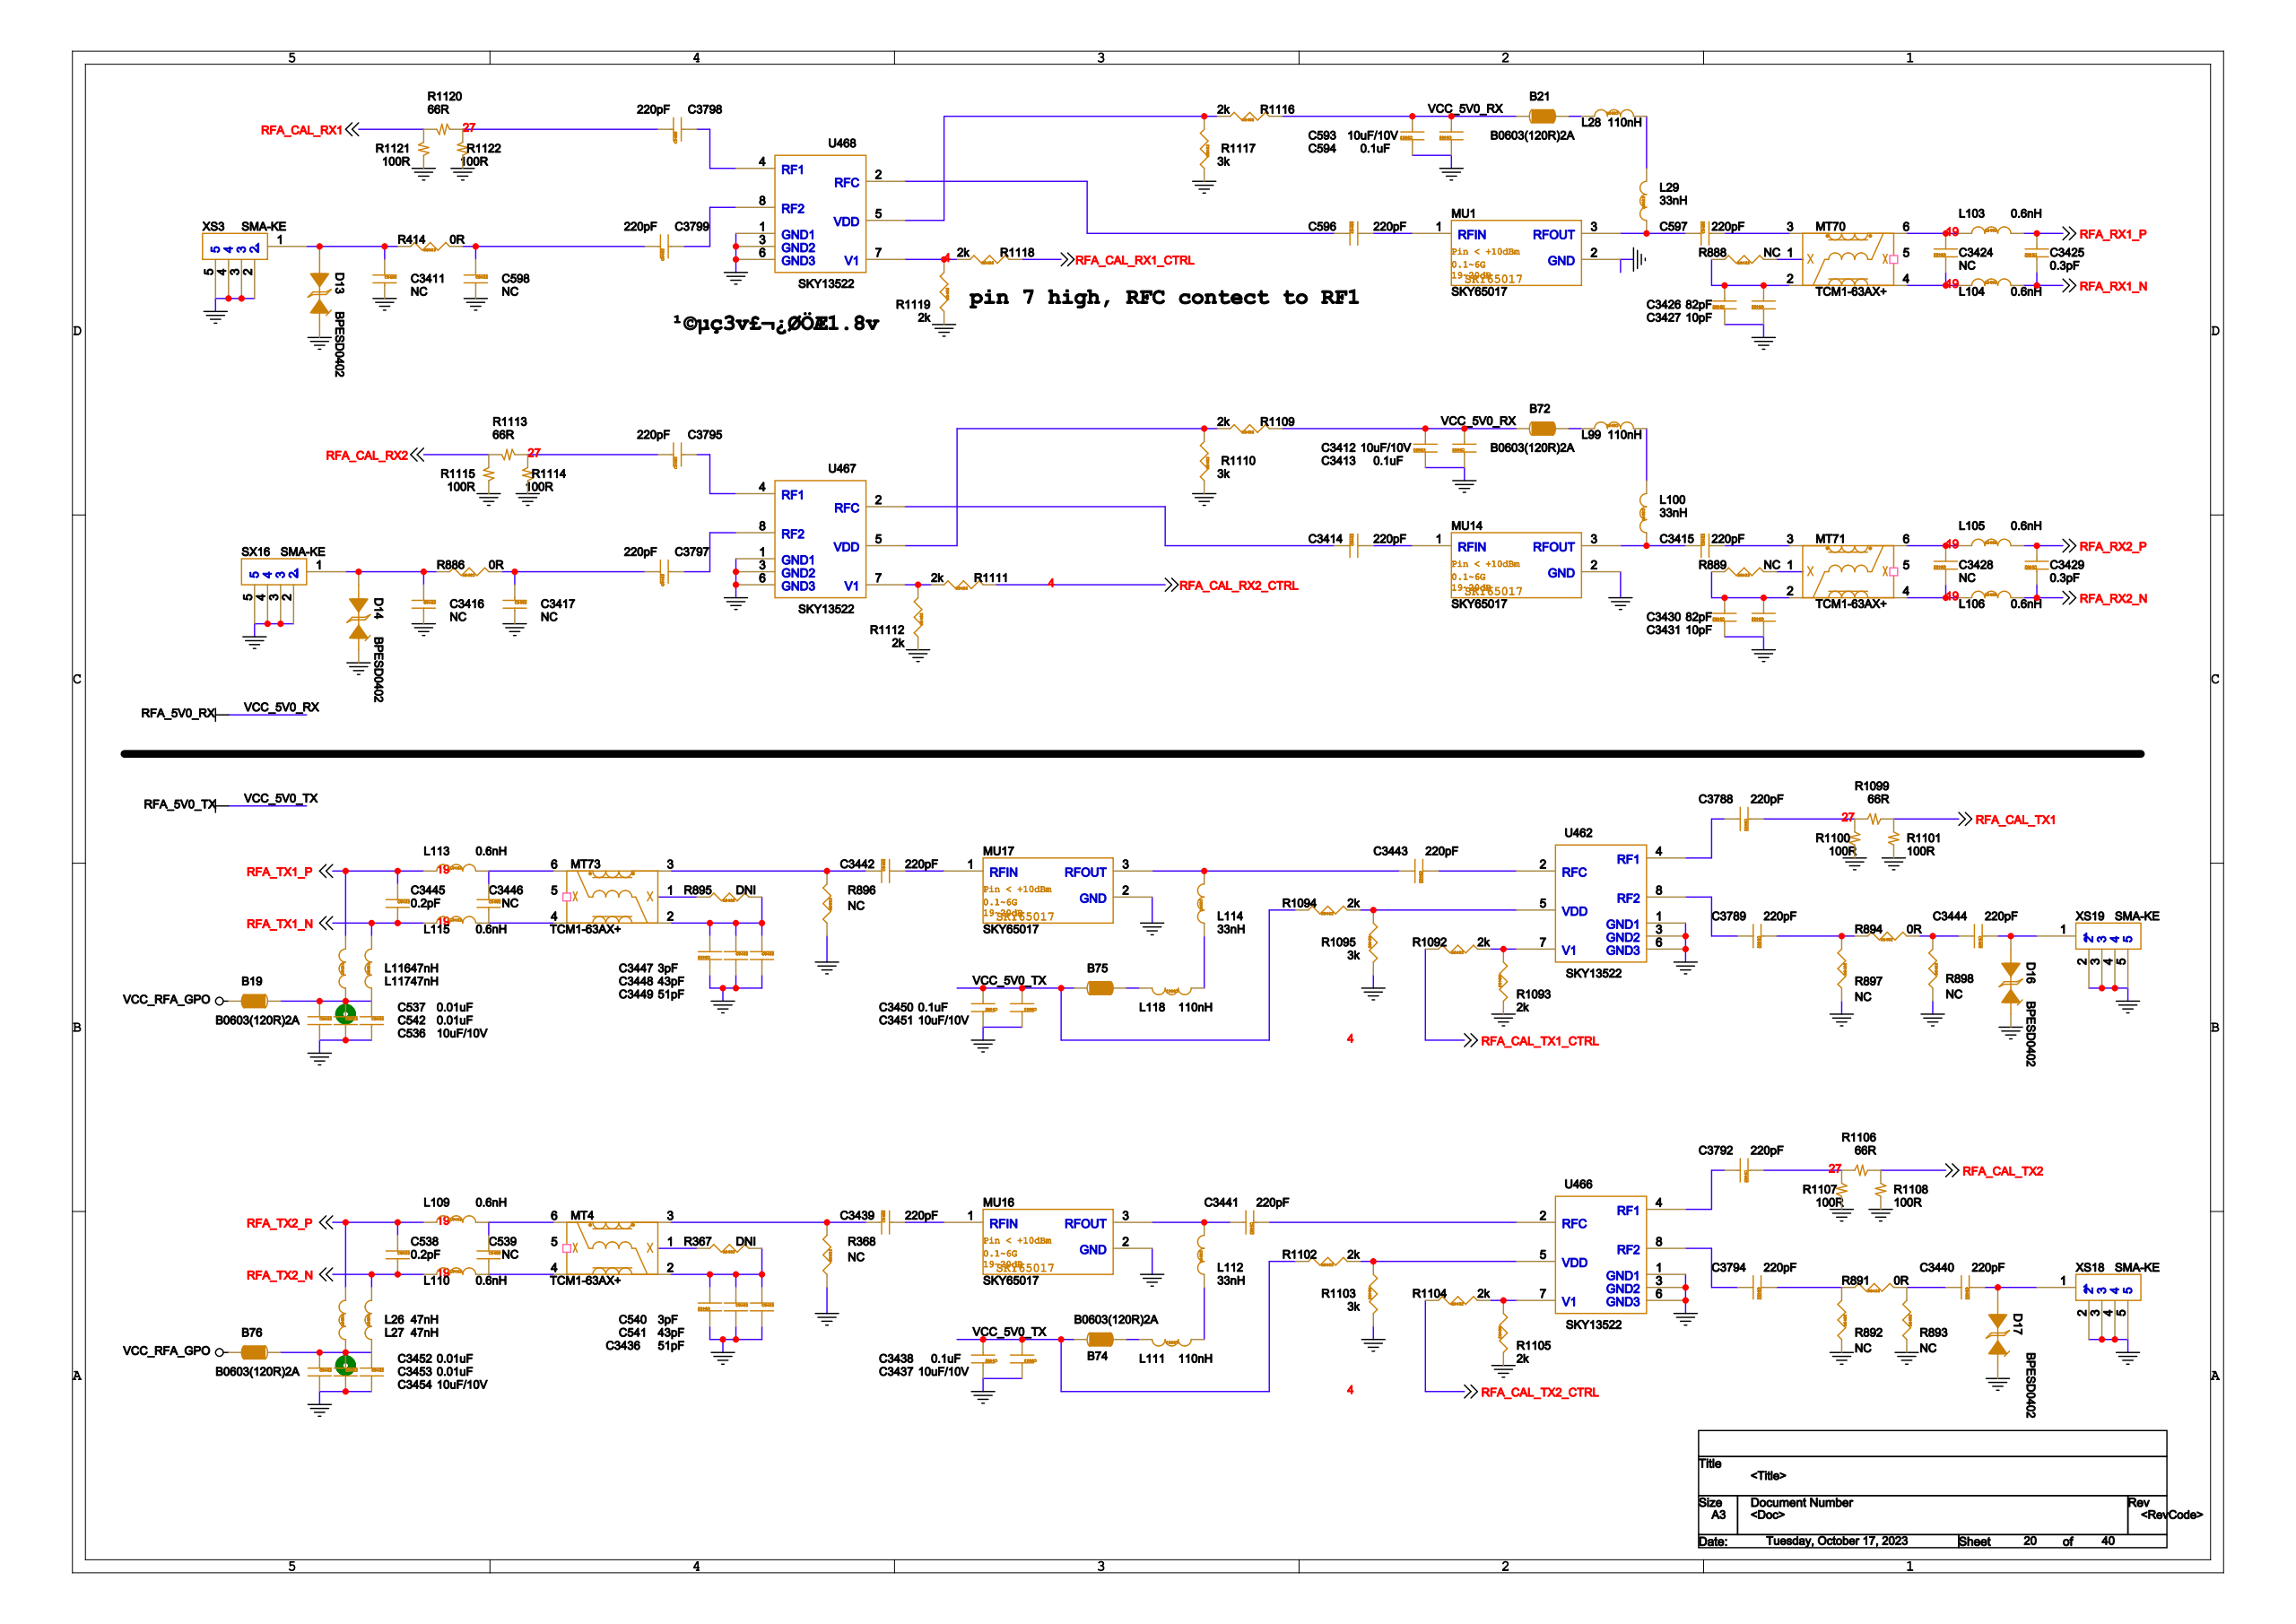Circuit board | Cadence Allegro | 1793 parts | 1223 nets | one sheet of the schematic
Parts on this sheet (reference | value | footprint):
B19 | B0603(120R)2A | B0603
B21 | B0603(120R)2A | B0603
B72 | B0603(120R)2A | B0603
B74 | B0603(120R)2A | B0603
B75 | B0603(120R)2A | B0603
B76 | B0603(120R)2A | B0603
C536 | 10uF/10V | C0402
C537 | 0.01uF | C0402
C538 | 0.2pF | C0402
C539 | NC | C0402
C540 | 3pF | C0402
C541 | 43pF | C0402
C542 | 0.01uF | C0402
C593 | 10uF/10V | C0402
C594 | 0.1uF | C0402
C596 | 220pF | C0402
C597 | 220pF | C0402
C598 | NC | C0402
C3411 | NC | C0402
C3412 | 10uF/10V | C0402
C3413 | 0.1uF | C0402
C3414 | 220pF | C0402
C3415 | 220pF | C0402
C3416 | NC | C0402
C3417 | NC | C0402
C3424 | NC | C0402
C3425 | 0.3pF | C0402
C3426 | 82pF | C0402
C3427 | 10pF | C0402
C3428 | NC | C0402
C3429 | 0.3pF | C0402
C3430 | 82pF | C0402
C3431 | 10pF | C0402
C3436 | 51pF | C0402
C3437 | 10uF/10V | C0402
C3438 | 0.1uF | C0402
C3439 | 220pF | C0402
C3440 | 220pF | C0402
C3441 | 220pF | C0402
C3442 | 220pF | C0402
C3443 | 220pF | C0402
C3444 | 220pF | C0402
C3445 | 0.2pF | C0402
C3446 | NC | C0402
C3447 | 3pF | C0402
C3448 | 43pF | C0402
C3449 | 51pF | C0402
C3450 | 0.1uF | C0402
C3451 | 10uF/10V | C0402
C3452 | 0.01uF | C0402
C3453 | 0.01uF | C0402
C3454 | 10uF/10V | C0402
C3788 | 220pF | C0402
C3789 | 220pF | C0402
C3792 | 220pF | C0402
C3794 | 220pF | C0402
C3795 | 220pF | C0402
C3797 | 220pF | C0402
C3798 | 220pF | C0402
C3799 | 220pF | C0402
D13 | BPESD0402 | C0402
D14 | BPESD0402 | C0402
D16 | BPESD0402 | C0402
D17 | BPESD0402 | C0402
L26 | 47nH | L0603
L27 | 47nH | L0603
L28 | 110nH | L0603
L29 | 33nH | L0603
L99 | 110nH | L0603
L100 | 33nH | L0603
L103 | 0.6nH | L0402
L104 | 0.6nH | L0402
L105 | 0.6nH | L0402
L106 | 0.6nH | L0402
L109 | 0.6nH | L0402
L110 | 0.6nH | L0402
L111 | 110nH | L0603
L112 | 33nH | L0603
L113 | 0.6nH | L0402
L114 | 33nH | L0603
L115 | 0.6nH | L0402
L118 | 110nH | L0603
MT4 | TCM1-63AX+ | TCM1-63AX
MT70 | TCM1-63AX+ | TCM1-63AX
MT71 | TCM1-63AX+ | TCM1-63AX
MT73 | TCM1-63AX+ | TCM1-63AX
MU1 | SKY65017 | SOT89_3
MU14 | SKY65017 | SOT89_3
MU16 | SKY65017 | SOT89_3
MU17 | SKY65017 | SOT89_3
R367 | DNI | R0402
R368 | NC | R0402
R414 | 0R | R0603
R886 | 0R | R0603
R888 | NC | R0402
R889 | NC | R0402
R891 | 0R | R0402
R892 | NC | R0402
R893 | NC | R0402
R894 | 0R | R0402
R895 | DNI | R0402
R896 | NC | R0402
R897 | NC | R0402
R898 | NC | R0402
R1092 | 2k | R0402
R1093 | 2k | R0402
R1094 | 2k | R0402
R1095 | 3k | R0402
R1099 | 66R | R0402
R1100 | 100R | R0402
R1101 | 100R | R0402
R1102 | 2k | R0402
R1103 | 3k | R0402
R1104 | 2k | R0402
R1105 | 2k | R0402
R1106 | 66R | R0402
R1107 | 100R | R0402
R1108 | 100R | R0402
R1109 | 2k | R0402
R1110 | 3k | R0402
R1111 | 2k | R0402
R1112 | 2k | R0402
R1113 | 66R | R0402
R1114 | 100R | R0402
R1115 | 100R | R0402
R1116 | 2k | R0402
R1117 | 3k | R0402
R1118 | 2k | R0402
R1119 | 2k | R0402
R1120 | 66R | R0402
R1121 | 100R | R0402
R1122 | 100R | R0402
SX16 | SMA-KE | SMA-SMD_BWSMA-KE-P001
U462 | SKY13522 | TSNP-8_L1_1-W1_1-P0_40-BL
U466 | SKY13522 | TSNP-8_L1_1-W1_1-P0_40-BL
U467 | SKY13522 | TSNP-8_L1_1-W1_1-P0_40-BL
U468 | SKY13522 | TSNP-8_L1_1-W1_1-P0_40-BL
XS3 | SMA-KE | SMA-SMD_BWSMA-KE-P001
XS18 | SMA-KE | SMA-SMD_BWSMA-KE-P001
XS19 | SMA-KE | SMA-SMD_BWSMA-KE-P001
Nets of these parts (net: part-pin ...):
GND: C536-2 C537-2 C540-1 C541-2 C542-2 C593-1 C594-1 C598-2 C3411-2 C3412-1 C3413-1 C3416-2 C3417-2 C3426-1 C3427-1 C3430-1 C3431-1 C3436-2 C3437-1 C3438-1 C3447-1 C3448-2 C3449-2 C3450-1 C3451-1 C3452-2 C3453-2 C3454-2 D13-2 D14-2 D16-2 D17-2 MU1-2 MU14-2 MU16-2 MU17-2 R368-1 R892-1 R893-1 R896-1 R897-1 R898-1 R1093-2 R1095-2 R1100-1 R1101-1 R1103-2 R1105-2 R1107-1 R1108-1 R1110-2 R1112-2 R1114-1 R1115-1 R1117-2 R1119-2 R1121-1 R1122-1 SX16-2 SX16-3 SX16-4 SX16-5 U462-1 U462-3 U462-6 U466-1 U466-3 U466-6 U467-1 U467-3 U467-6 U468-1 U468-3 U468-6 XS3-2 XS3-3 XS3-4 XS3-5 XS18-2 XS18-3 XS18-4 XS18-5 XS19-2 XS19-3 XS19-4 XS19-5
N17038594: C3411-1 D13-1 R414-1 XS3-1
N17042265: C3416-1 D14-1 R886-1 SX16-1
N17055895: C3444-1 D16-1 XS19-1
N17056237: C3440-1 D17-1 XS18-1
RFA_CAL_TX1_CTRL: R1092-1
N18637396: R1092-2 R1093-1 U462-7
RFA_5V0_TX: B74-1 B75-1 C3437-2 C3438-2 C3450-2 C3451-2 R1094-1 R1102-1
N18612424: R1094-2 R1095-1 U462-5
N18679446: R1102-2 R1103-1 U466-5
RFA_CAL_TX2_CTRL: R1104-1
N18679484: R1104-2 R1105-1 U466-7
RFA_5V0_RX: B21-1 B72-1 C593-2 C594-2 C3412-2 C3413-2 R1109-1 R1116-1
N18681713: R1109-2 R1110-1 U467-5
RFA_CAL_RX2_CTRL: R1111-1
N18681751: R1111-2 R1112-1 U467-7
N18683006: R1116-2 R1117-1 U468-5
RFA_CAL_RX1_CTRL: R1118-1
N18683048: R1118-2 R1119-1 U468-7
N18664130: C3788-1 R1099-1 R1100-2
RFA_CAL_TX1: R1099-2 R1101-2
N18679400: C3792-1 R1106-1 R1107-2
RFA_CAL_TX2: R1106-2 R1108-2
N18681669: C3795-1 R1113-1 R1114-2
RFA_CAL_RX2: R1113-2 R1115-2
N18682970: C3798-1 R1120-1 R1122-2
RFA_CAL_RX1: R1120-2 R1121-2
N18612280: C3788-2 U462-4
N18664648: C3789-2 U462-8
N18612132: C3443-1 U462-2
N18679396: C3792-2 U466-4
N18679438: C3794-2 U466-8
N18679426: C3441-1 U466-2
N18681665: C3795-2 U467-4
N18681707: C3797-2 U467-8
N18681695: C3414-1 U467-2
N18682972: C3798-2 U468-4
N18682994: C3799-2 U468-8
N18682992: C596-1 U468-2
N17056451: B76-1 C3452-1 C3453-1 C3454-1 L26-1 L27-1
N17056106: B19-1 C536-1 C537-1 C542-1
N17038892: C596-2 MU1-1
N1059479: C597-1 L29-2 MU1-3
N17042279: C3414-2 MU14-1
N17042281: C3415-1 L100-2 MU14-3
N17056223: C3439-2 MU16-1
N17056225: C3441-2 L112-1 MU16-3
N17055881: C3442-2 MU17-1
N17055883: C3443-2 L114-1 MU17-3
RFA_RX1_N: C3425-1 L104-2
RFA_RX1_P: C3425-2 L103-2
RFA_RX2_N: C3429-1 L106-2
RFA_RX2_P: C3429-2 L105-2
RFA_TX1_N: C3445-2 L115-1
RFA_TX1_P: C3445-1 L113-1
RFA_TX2_N: C538-2 L27-2 L110-1
RFA_TX2_P: C538-1 L26-2 L109-1
VCC_RFA_GPO: B19-2 B76-2
N17039097: B21-2 L28-2
N17042195: B72-2 L99-2
N17056438: B74-2 L111-2
N17056096: B75-2 L118-2
N17042273: C3417-1 C3797-1 R886-2
N17042946: C3424-1 L104-1 MT70-4
N17042909: C3424-2 L103-1 MT70-6
N17044828: C3428-1 L106-1 MT71-4
N17044794: C3428-2 L105-1 MT71-6
N17055861: C3446-1 L113-2 MT73-6
N17055984: C3446-2 L115-2 MT73-4
N17056203: C539-1 L109-2 MT4-6
N17056326: C539-2 L110-2 MT4-4
N724433: C598-1 C3799-1 R414-2
N17055889: C3789-1 R894-1 R897-2
N17056229: C3794-1 R891-1 R892-2
N17044780: C3415-2 MT71-3
N17056219: C3439-1 MT4-3 R368-2
N17056235: C3440-2 R891-2 R893-2
N17055877: C3442-1 MT73-3 R896-2
N17055891: C3444-2 R894-2 R898-2
N1025474: C597-2 MT70-3
N17042942: C3426-2 C3427-2 MT70-2 R888-1
N17044824: C3430-2 C3431-2 MT71-2 R889-1
N17056301: C540-2 C541-1 C3436-1 MT4-2 R367-2
N17055959: C3447-2 C3448-1 C3449-1 MT73-2 R895-2
N17042197: L99-1 L100-1
N17056344: L111-1 L112-2
N17056002: L114-2 L118-1
N17039045: L28-1 L29-1
N17056299: MT4-1 R367-1
N17042944: MT70-1 R888-2
N17044826: MT71-1 R889-2
N17055957: MT73-1 R895-1